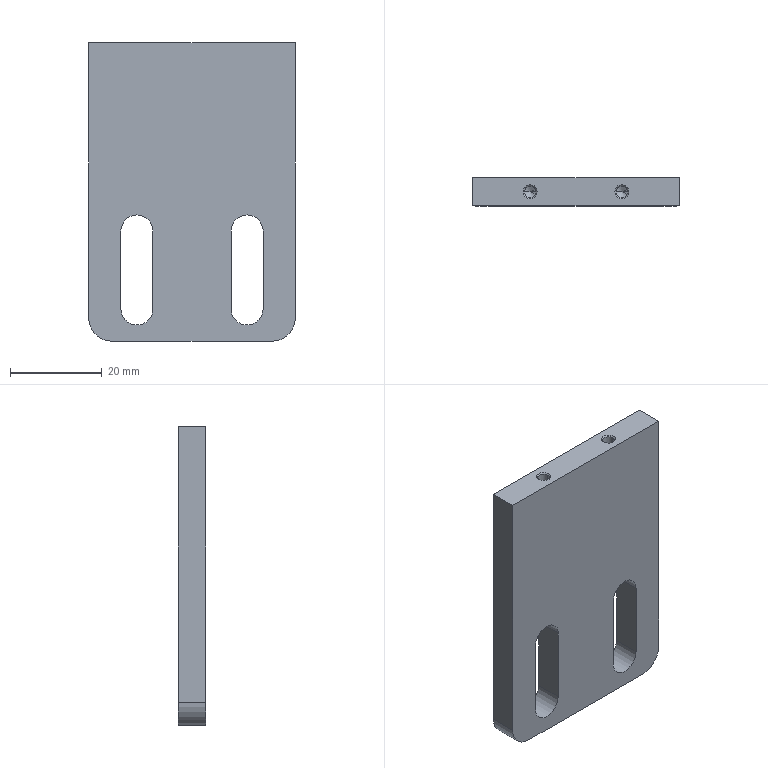Part | SolidWorks | features Extrusion 1, Fillet 1, HoleWzd 1, ICE 1 | 1 solid | 30 faces | box 45 x 6 x 65 mm | volume 15460 mm3 | cylinder 12 | plane 10 | cone 8 | commonest cylinder face diameters 7 x6 2.5 x4 10 x2
STEP:
#1=CARTESIAN_POINT('',(-11.25,3.,32.225));
#2=VERTEX_POINT('',#1);
#3=CARTESIAN_POINT('',(-8.75,3.,32.225));
#4=VERTEX_POINT('',#3);
#5=CARTESIAN_POINT('',(-10.,3.,32.225));
#6=DIRECTION('',(0.,0.,1.));
#7=DIRECTION('',(1.,0.,0.));
#8=AXIS2_PLACEMENT_3D('',#5,#6,#7);
#9=CIRCLE('',#8,1.25);
#10=EDGE_CURVE('',#2,#4,#9,.T.);
#11=ORIENTED_EDGE('',*,*,#10,.F.);
#12=CARTESIAN_POINT('',(-11.525,3.,32.5));
#13=VERTEX_POINT('',#12);
#14=CARTESIAN_POINT('',(-11.525,3.,32.5));
#15=DIRECTION('',(-0.7071,0.,0.7071));
#16=VECTOR('',#15,1000.);
#17=LINE('',#14,#16);
#18=EDGE_CURVE('',#2,#13,#17,.T.);
#19=ORIENTED_EDGE('',*,*,#18,.T.);
#20=CARTESIAN_POINT('',(-8.475,3.,32.5));
#21=VERTEX_POINT('',#20);
#22=CARTESIAN_POINT('',(-10.,3.,32.5));
#23=DIRECTION('',(0.,0.,1.));
#24=DIRECTION('',(1.,0.,0.));
#25=AXIS2_PLACEMENT_3D('',#22,#23,#24);
#26=CIRCLE('',#25,1.525);
#27=EDGE_CURVE('',#13,#21,#26,.T.);
#28=ORIENTED_EDGE('',*,*,#27,.T.);
#29=CARTESIAN_POINT('',(-8.475,3.,32.5));
#30=DIRECTION('',(0.7071,0.,0.7071));
#31=VECTOR('',#30,1000.);
#32=LINE('',#29,#31);
#33=EDGE_CURVE('',#4,#21,#32,.T.);
#34=ORIENTED_EDGE('',*,*,#33,.F.);
#35=EDGE_LOOP('',(#11,#19,#28,#34));
#36=FACE_OUTER_BOUND('',#35,.T.);
#37=CARTESIAN_POINT('',(-10.,3.,32.5));
#38=DIRECTION('',(0.,0.,1.));
#39=DIRECTION('',(1.,0.,0.));
#40=AXIS2_PLACEMENT_3D('',#37,#38,#39);
#41=CONICAL_SURFACE('',#40,1.525,0.7854);
#42=ADVANCED_FACE('',(#36),#41,.F.);
#43=CARTESIAN_POINT('',(-11.25,3.,19.));
#44=VERTEX_POINT('',#43);
#45=CARTESIAN_POINT('',(-8.75,3.,19.));
#46=VERTEX_POINT('',#45);
#47=CARTESIAN_POINT('',(-10.,3.,19.));
#48=DIRECTION('',(0.,0.,1.));
#49=DIRECTION('',(1.,0.,0.));
#50=AXIS2_PLACEMENT_3D('',#47,#48,#49);
#51=CIRCLE('',#50,1.25);
#52=EDGE_CURVE('',#44,#46,#51,.T.);
#53=ORIENTED_EDGE('',*,*,#52,.F.);
#54=CARTESIAN_POINT('',(-11.25,3.,32.5));
#55=DIRECTION('',(0.,0.,1.));
#56=VECTOR('',#55,1000.);
#57=LINE('',#54,#56);
#58=EDGE_CURVE('',#44,#2,#57,.T.);
#59=ORIENTED_EDGE('',*,*,#58,.T.);
#60=ORIENTED_EDGE('',*,*,#10,.T.);
#61=CARTESIAN_POINT('',(-8.75,3.,32.5));
#62=DIRECTION('',(0.,0.,1.));
#63=VECTOR('',#62,1000.);
#64=LINE('',#61,#63);
#65=EDGE_CURVE('',#46,#4,#64,.T.);
#66=ORIENTED_EDGE('',*,*,#65,.F.);
#67=EDGE_LOOP('',(#53,#59,#60,#66));
#68=FACE_OUTER_BOUND('',#67,.T.);
#69=CARTESIAN_POINT('',(-10.,3.,32.5));
#70=DIRECTION('',(0.,0.,1.));
#71=DIRECTION('',(1.,0.,0.));
#72=AXIS2_PLACEMENT_3D('',#69,#70,#71);
#73=CYLINDRICAL_SURFACE('',#72,1.25);
#74=ADVANCED_FACE('',(#68),#73,.F.);
#75=CARTESIAN_POINT('',(-10.,3.,18.249));
#76=VERTEX_POINT('',#75);
#77=CARTESIAN_POINT('',(-8.75,3.,19.));
#78=DIRECTION('',(0.8572,0.,0.515));
#79=VECTOR('',#78,1000.);
#80=LINE('',#77,#79);
#81=EDGE_CURVE('',#76,#46,#80,.T.);
#82=ORIENTED_EDGE('',*,*,#81,.F.);
#83=CARTESIAN_POINT('',(-11.25,3.,19.));
#84=DIRECTION('',(-0.8572,0.,0.515));
#85=VECTOR('',#84,1000.);
#86=LINE('',#83,#85);
#87=EDGE_CURVE('',#76,#44,#86,.T.);
#88=ORIENTED_EDGE('',*,*,#87,.T.);
#89=ORIENTED_EDGE('',*,*,#52,.T.);
#90=EDGE_LOOP('',(#82,#88,#89));
#91=FACE_OUTER_BOUND('',#90,.T.);
#92=CARTESIAN_POINT('',(-10.,3.,19.));
#93=DIRECTION('',(0.,0.,1.));
#94=DIRECTION('',(1.,0.,0.));
#95=AXIS2_PLACEMENT_3D('',#92,#93,#94);
#96=CONICAL_SURFACE('',#95,1.25,1.03);
#97=ADVANCED_FACE('',(#91),#96,.F.);
#98=CARTESIAN_POINT('',(8.75,3.,32.225));
#99=VERTEX_POINT('',#98);
#100=CARTESIAN_POINT('',(11.25,3.,32.225));
#101=VERTEX_POINT('',#100);
#102=CARTESIAN_POINT('',(10.,3.,32.225));
#103=DIRECTION('',(0.,0.,1.));
#104=DIRECTION('',(1.,0.,0.));
#105=AXIS2_PLACEMENT_3D('',#102,#103,#104);
#106=CIRCLE('',#105,1.25);
#107=EDGE_CURVE('',#99,#101,#106,.T.);
#108=ORIENTED_EDGE('',*,*,#107,.F.);
#109=CARTESIAN_POINT('',(8.475,3.,32.5));
#110=VERTEX_POINT('',#109);
#111=CARTESIAN_POINT('',(8.475,3.,32.5));
#112=DIRECTION('',(-0.7071,0.,0.7071));
#113=VECTOR('',#112,1000.);
#114=LINE('',#111,#113);
#115=EDGE_CURVE('',#99,#110,#114,.T.);
#116=ORIENTED_EDGE('',*,*,#115,.T.);
#117=CARTESIAN_POINT('',(11.525,3.,32.5));
#118=VERTEX_POINT('',#117);
#119=CARTESIAN_POINT('',(10.,3.,32.5));
#120=DIRECTION('',(0.,0.,1.));
#121=DIRECTION('',(1.,0.,0.));
#122=AXIS2_PLACEMENT_3D('',#119,#120,#121);
#123=CIRCLE('',#122,1.525);
#124=EDGE_CURVE('',#110,#118,#123,.T.);
#125=ORIENTED_EDGE('',*,*,#124,.T.);
#126=CARTESIAN_POINT('',(11.525,3.,32.5));
#127=DIRECTION('',(0.7071,0.,0.7071));
#128=VECTOR('',#127,1000.);
#129=LINE('',#126,#128);
#130=EDGE_CURVE('',#101,#118,#129,.T.);
#131=ORIENTED_EDGE('',*,*,#130,.F.);
#132=EDGE_LOOP('',(#108,#116,#125,#131));
#133=FACE_OUTER_BOUND('',#132,.T.);
#134=CARTESIAN_POINT('',(10.,3.,32.5));
#135=DIRECTION('',(0.,0.,1.));
#136=DIRECTION('',(1.,0.,0.));
#137=AXIS2_PLACEMENT_3D('',#134,#135,#136);
#138=CONICAL_SURFACE('',#137,1.525,0.7854);
#139=ADVANCED_FACE('',(#133),#138,.F.);
#140=CARTESIAN_POINT('',(8.75,3.,19.));
#141=VERTEX_POINT('',#140);
#142=CARTESIAN_POINT('',(11.25,3.,19.));
#143=VERTEX_POINT('',#142);
#144=CARTESIAN_POINT('',(10.,3.,19.));
#145=DIRECTION('',(0.,0.,1.));
#146=DIRECTION('',(1.,0.,0.));
#147=AXIS2_PLACEMENT_3D('',#144,#145,#146);
#148=CIRCLE('',#147,1.25);
#149=EDGE_CURVE('',#141,#143,#148,.T.);
#150=ORIENTED_EDGE('',*,*,#149,.F.);
#151=CARTESIAN_POINT('',(8.75,3.,32.5));
#152=DIRECTION('',(0.,0.,1.));
#153=VECTOR('',#152,1000.);
#154=LINE('',#151,#153);
#155=EDGE_CURVE('',#141,#99,#154,.T.);
#156=ORIENTED_EDGE('',*,*,#155,.T.);
#157=ORIENTED_EDGE('',*,*,#107,.T.);
#158=CARTESIAN_POINT('',(11.25,3.,32.5));
#159=DIRECTION('',(0.,0.,1.));
#160=VECTOR('',#159,1000.);
#161=LINE('',#158,#160);
#162=EDGE_CURVE('',#143,#101,#161,.T.);
#163=ORIENTED_EDGE('',*,*,#162,.F.);
#164=EDGE_LOOP('',(#150,#156,#157,#163));
#165=FACE_OUTER_BOUND('',#164,.T.);
#166=CARTESIAN_POINT('',(10.,3.,32.5));
#167=DIRECTION('',(0.,0.,1.));
#168=DIRECTION('',(1.,0.,0.));
#169=AXIS2_PLACEMENT_3D('',#166,#167,#168);
#170=CYLINDRICAL_SURFACE('',#169,1.25);
#171=ADVANCED_FACE('',(#165),#170,.F.);
#172=CARTESIAN_POINT('',(10.,3.,18.249));
#173=VERTEX_POINT('',#172);
#174=CARTESIAN_POINT('',(11.25,3.,19.));
#175=DIRECTION('',(0.8572,0.,0.515));
#176=VECTOR('',#175,1000.);
#177=LINE('',#174,#176);
#178=EDGE_CURVE('',#173,#143,#177,.T.);
#179=ORIENTED_EDGE('',*,*,#178,.F.);
#180=CARTESIAN_POINT('',(8.75,3.,19.));
#181=DIRECTION('',(-0.8572,0.,0.515));
#182=VECTOR('',#181,1000.);
#183=LINE('',#180,#182);
#184=EDGE_CURVE('',#173,#141,#183,.T.);
#185=ORIENTED_EDGE('',*,*,#184,.T.);
#186=ORIENTED_EDGE('',*,*,#149,.T.);
#187=EDGE_LOOP('',(#179,#185,#186));
#188=FACE_OUTER_BOUND('',#187,.T.);
#189=CARTESIAN_POINT('',(10.,3.,19.));
#190=DIRECTION('',(0.,0.,1.));
#191=DIRECTION('',(1.,0.,0.));
#192=AXIS2_PLACEMENT_3D('',#189,#190,#191);
#193=CONICAL_SURFACE('',#192,1.25,1.03);
#194=ADVANCED_FACE('',(#188),#193,.F.);
#195=CARTESIAN_POINT('',(-12.,0.,-5.));
#196=VERTEX_POINT('',#195);
#197=CARTESIAN_POINT('',(-8.5,0.,-8.5));
#198=VERTEX_POINT('',#197);
#199=CARTESIAN_POINT('',(-12.,0.,-8.5));
#200=DIRECTION('',(0.,1.,0.));
#201=DIRECTION('',(0.,0.,1.));
#202=AXIS2_PLACEMENT_3D('',#199,#200,#201);
#203=CIRCLE('',#202,3.5);
#204=EDGE_CURVE('',#196,#198,#203,.T.);
#205=ORIENTED_EDGE('',*,*,#204,.F.);
#206=CARTESIAN_POINT('',(-12.,6.,-5.));
#207=VERTEX_POINT('',#206);
#208=CARTESIAN_POINT('',(-12.,0.,-5.));
#209=DIRECTION('',(0.,1.,0.));
#210=VECTOR('',#209,1000.);
#211=LINE('',#208,#210);
#212=EDGE_CURVE('',#196,#207,#211,.T.);
#213=ORIENTED_EDGE('',*,*,#212,.T.);
#214=CARTESIAN_POINT('',(-8.5,6.,-8.5));
#215=VERTEX_POINT('',#214);
#216=CARTESIAN_POINT('',(-12.,6.,-8.5));
#217=DIRECTION('',(0.,1.,0.));
#218=DIRECTION('',(0.,0.,1.));
#219=AXIS2_PLACEMENT_3D('',#216,#217,#218);
#220=CIRCLE('',#219,3.5);
#221=EDGE_CURVE('',#207,#215,#220,.T.);
#222=ORIENTED_EDGE('',*,*,#221,.T.);
#223=CARTESIAN_POINT('',(-8.5,0.,-8.5));
#224=DIRECTION('',(0.,1.,0.));
#225=VECTOR('',#224,1000.);
#226=LINE('',#223,#225);
#227=EDGE_CURVE('',#198,#215,#226,.T.);
#228=ORIENTED_EDGE('',*,*,#227,.F.);
#229=EDGE_LOOP('',(#205,#213,#222,#228));
#230=FACE_OUTER_BOUND('',#229,.T.);
#231=CARTESIAN_POINT('',(-12.,0.,-8.5));
#232=DIRECTION('',(0.,1.,0.));
#233=DIRECTION('',(0.,0.,1.));
#234=AXIS2_PLACEMENT_3D('',#231,#232,#233);
#235=CYLINDRICAL_SURFACE('',#234,3.5);
#236=ADVANCED_FACE('',(#230),#235,.F.);
#237=CARTESIAN_POINT('',(12.,0.,-5.));
#238=VERTEX_POINT('',#237);
#239=CARTESIAN_POINT('',(15.5,0.,-8.5));
#240=VERTEX_POINT('',#239);
#241=CARTESIAN_POINT('',(12.,0.,-8.5));
#242=DIRECTION('',(0.,1.,0.));
#243=DIRECTION('',(0.,0.,-1.));
#244=AXIS2_PLACEMENT_3D('',#241,#242,#243);
#245=CIRCLE('',#244,3.5);
#246=EDGE_CURVE('',#238,#240,#245,.T.);
#247=ORIENTED_EDGE('',*,*,#246,.F.);
#248=CARTESIAN_POINT('',(12.,6.,-5.));
#249=VERTEX_POINT('',#248);
#250=CARTESIAN_POINT('',(12.,0.,-5.));
#251=DIRECTION('',(0.,1.,0.));
#252=VECTOR('',#251,1000.);
#253=LINE('',#250,#252);
#254=EDGE_CURVE('',#238,#249,#253,.T.);
#255=ORIENTED_EDGE('',*,*,#254,.T.);
#256=CARTESIAN_POINT('',(15.5,6.,-8.5));
#257=VERTEX_POINT('',#256);
#258=CARTESIAN_POINT('',(12.,6.,-8.5));
#259=DIRECTION('',(0.,1.,0.));
#260=DIRECTION('',(0.,0.,-1.));
#261=AXIS2_PLACEMENT_3D('',#258,#259,#260);
#262=CIRCLE('',#261,3.5);
#263=EDGE_CURVE('',#249,#257,#262,.T.);
#264=ORIENTED_EDGE('',*,*,#263,.T.);
#265=CARTESIAN_POINT('',(15.5,0.,-8.5));
#266=DIRECTION('',(0.,1.,0.));
#267=VECTOR('',#266,1000.);
#268=LINE('',#265,#267);
#269=EDGE_CURVE('',#240,#257,#268,.T.);
#270=ORIENTED_EDGE('',*,*,#269,.F.);
#271=EDGE_LOOP('',(#247,#255,#264,#270));
#272=FACE_OUTER_BOUND('',#271,.T.);
#273=CARTESIAN_POINT('',(12.,0.,-8.5));
#274=DIRECTION('',(0.,1.,0.));
#275=DIRECTION('',(0.,0.,1.));
#276=AXIS2_PLACEMENT_3D('',#273,#274,#275);
#277=CYLINDRICAL_SURFACE('',#276,3.5);
#278=ADVANCED_FACE('',(#272),#277,.F.);
#279=CARTESIAN_POINT('',(-22.5,6.,-27.5));
#280=VERTEX_POINT('',#279);
#281=CARTESIAN_POINT('',(-22.5,6.,32.5));
#282=VERTEX_POINT('',#281);
#283=CARTESIAN_POINT('',(-22.5,6.,32.5));
#284=DIRECTION('',(0.,0.,1.));
#285=VECTOR('',#284,1000.);
#286=LINE('',#283,#285);
#287=EDGE_CURVE('',#280,#282,#286,.T.);
#288=ORIENTED_EDGE('',*,*,#287,.F.);
#289=CARTESIAN_POINT('',(-22.5,0.,-27.5));
#290=VERTEX_POINT('',#289);
#291=CARTESIAN_POINT('',(-22.5,6.,-27.5));
#292=DIRECTION('',(0.,-1.,0.));
#293=VECTOR('',#292,1000.);
#294=LINE('',#291,#293);
#295=EDGE_CURVE('',#280,#290,#294,.T.);
#296=ORIENTED_EDGE('',*,*,#295,.T.);
#297=CARTESIAN_POINT('',(-22.5,0.,32.5));
#298=VERTEX_POINT('',#297);
#299=CARTESIAN_POINT('',(-22.5,0.,32.5));
#300=DIRECTION('',(0.,0.,1.));
#301=VECTOR('',#300,1000.);
#302=LINE('',#299,#301);
#303=EDGE_CURVE('',#290,#298,#302,.T.);
#304=ORIENTED_EDGE('',*,*,#303,.T.);
#305=CARTESIAN_POINT('',(-22.5,6.,32.5));
#306=DIRECTION('',(0.,-1.,0.));
#307=VECTOR('',#306,1000.);
#308=LINE('',#305,#307);
#309=EDGE_CURVE('',#282,#298,#308,.T.);
#310=ORIENTED_EDGE('',*,*,#309,.F.);
#311=EDGE_LOOP('',(#288,#296,#304,#310));
#312=FACE_OUTER_BOUND('',#311,.T.);
#313=CARTESIAN_POINT('',(-22.5,6.,32.5));
#314=DIRECTION('',(1.,0.,0.));
#315=DIRECTION('',(0.,0.,-1.));
#316=AXIS2_PLACEMENT_3D('',#313,#314,#315);
#317=PLANE('',#316);
#318=ADVANCED_FACE('',(#312),#317,.F.);
#319=CARTESIAN_POINT('',(-10.,3.,32.5));
#320=DIRECTION('',(0.,0.,1.));
#321=DIRECTION('',(1.,0.,0.));
#322=AXIS2_PLACEMENT_3D('',#319,#320,#321);
#323=CIRCLE('',#322,1.525);
#324=EDGE_CURVE('',#21,#13,#323,.T.);
#325=ORIENTED_EDGE('',*,*,#324,.F.);
#326=ORIENTED_EDGE('',*,*,#27,.F.);
#327=EDGE_LOOP('',(#325,#326));
#328=FACE_BOUND('',#327,.T.);
#329=CARTESIAN_POINT('',(10.,3.,32.5));
#330=DIRECTION('',(0.,0.,1.));
#331=DIRECTION('',(1.,0.,0.));
#332=AXIS2_PLACEMENT_3D('',#329,#330,#331);
#333=CIRCLE('',#332,1.525);
#334=EDGE_CURVE('',#118,#110,#333,.T.);
#335=ORIENTED_EDGE('',*,*,#334,.F.);
#336=ORIENTED_EDGE('',*,*,#124,.F.);
#337=EDGE_LOOP('',(#335,#336));
#338=FACE_BOUND('',#337,.T.);
#339=CARTESIAN_POINT('',(22.5,0.,32.5));
#340=VERTEX_POINT('',#339);
#341=CARTESIAN_POINT('',(22.5,0.,32.5));
#342=DIRECTION('',(1.,0.,0.));
#343=VECTOR('',#342,1000.);
#344=LINE('',#341,#343);
#345=EDGE_CURVE('',#298,#340,#344,.T.);
#346=ORIENTED_EDGE('',*,*,#345,.T.);
#347=CARTESIAN_POINT('',(22.5,6.,32.5));
#348=VERTEX_POINT('',#347);
#349=CARTESIAN_POINT('',(22.5,6.,32.5));
#350=DIRECTION('',(0.,-1.,0.));
#351=VECTOR('',#350,1000.);
#352=LINE('',#349,#351);
#353=EDGE_CURVE('',#348,#340,#352,.T.);
#354=ORIENTED_EDGE('',*,*,#353,.F.);
#355=CARTESIAN_POINT('',(22.5,6.,32.5));
#356=DIRECTION('',(1.,0.,0.));
#357=VECTOR('',#356,1000.);
#358=LINE('',#355,#357);
#359=EDGE_CURVE('',#282,#348,#358,.T.);
#360=ORIENTED_EDGE('',*,*,#359,.F.);
#361=ORIENTED_EDGE('',*,*,#309,.T.);
#362=EDGE_LOOP('',(#346,#354,#360,#361));
#363=FACE_OUTER_BOUND('',#362,.T.);
#364=CARTESIAN_POINT('',(22.5,6.,32.5));
#365=DIRECTION('',(0.,0.,-1.));
#366=DIRECTION('',(-1.,0.,0.));
#367=AXIS2_PLACEMENT_3D('',#364,#365,#366);
#368=PLANE('',#367);
#369=ADVANCED_FACE('',(#328,#338,#363),#368,.F.);
#370=CARTESIAN_POINT('',(22.5,0.,-27.5));
#371=VERTEX_POINT('',#370);
#372=CARTESIAN_POINT('',(22.5,0.,32.5));
#373=DIRECTION('',(0.,0.,-1.));
#374=VECTOR('',#373,1000.);
#375=LINE('',#372,#374);
#376=EDGE_CURVE('',#340,#371,#375,.T.);
#377=ORIENTED_EDGE('',*,*,#376,.T.);
#378=CARTESIAN_POINT('',(22.5,6.,-27.5));
#379=VERTEX_POINT('',#378);
#380=CARTESIAN_POINT('',(22.5,6.,-27.5));
#381=DIRECTION('',(0.,1.,0.));
#382=VECTOR('',#381,1000.);
#383=LINE('',#380,#382);
#384=EDGE_CURVE('',#371,#379,#383,.T.);
#385=ORIENTED_EDGE('',*,*,#384,.T.);
#386=CARTESIAN_POINT('',(22.5,6.,32.5));
#387=DIRECTION('',(0.,0.,-1.));
#388=VECTOR('',#387,1000.);
#389=LINE('',#386,#388);
#390=EDGE_CURVE('',#348,#379,#389,.T.);
#391=ORIENTED_EDGE('',*,*,#390,.F.);
#392=ORIENTED_EDGE('',*,*,#353,.T.);
#393=EDGE_LOOP('',(#377,#385,#391,#392));
#394=FACE_OUTER_BOUND('',#393,.T.);
#395=CARTESIAN_POINT('',(22.5,6.,32.5));
#396=DIRECTION('',(-1.,0.,0.));
#397=DIRECTION('',(0.,0.,1.));
#398=AXIS2_PLACEMENT_3D('',#395,#396,#397);
#399=PLANE('',#398);
#400=ADVANCED_FACE('',(#394),#399,.F.);
#401=CARTESIAN_POINT('',(17.5,6.,-32.5));
#402=VERTEX_POINT('',#401);
#403=CARTESIAN_POINT('',(-17.5,6.,-32.5));
#404=VERTEX_POINT('',#403);
#405=CARTESIAN_POINT('',(22.5,6.,-32.5));
#406=DIRECTION('',(-1.,0.,0.));
#407=VECTOR('',#406,1000.);
#408=LINE('',#405,#407);
#409=EDGE_CURVE('',#402,#404,#408,.T.);
#410=ORIENTED_EDGE('',*,*,#409,.F.);
#411=CARTESIAN_POINT('',(17.5,0.,-32.5));
#412=VERTEX_POINT('',#411);
#413=CARTESIAN_POINT('',(17.5,6.,-32.5));
#414=DIRECTION('',(0.,-1.,0.));
#415=VECTOR('',#414,1000.);
#416=LINE('',#413,#415);
#417=EDGE_CURVE('',#402,#412,#416,.T.);
#418=ORIENTED_EDGE('',*,*,#417,.T.);
#419=CARTESIAN_POINT('',(-17.5,0.,-32.5));
#420=VERTEX_POINT('',#419);
#421=CARTESIAN_POINT('',(22.5,0.,-32.5));
#422=DIRECTION('',(-1.,0.,0.));
#423=VECTOR('',#422,1000.);
#424=LINE('',#421,#423);
#425=EDGE_CURVE('',#412,#420,#424,.T.);
#426=ORIENTED_EDGE('',*,*,#425,.T.);
#427=CARTESIAN_POINT('',(-17.5,6.,-32.5));
#428=DIRECTION('',(0.,1.,0.));
#429=VECTOR('',#428,1000.);
#430=LINE('',#427,#429);
#431=EDGE_CURVE('',#420,#404,#430,.T.);
#432=ORIENTED_EDGE('',*,*,#431,.T.);
#433=EDGE_LOOP('',(#410,#418,#426,#432));
#434=FACE_OUTER_BOUND('',#433,.T.);
#435=CARTESIAN_POINT('',(22.5,6.,-32.5));
#436=DIRECTION('',(0.,0.,1.));
#437=DIRECTION('',(1.,0.,0.));
#438=AXIS2_PLACEMENT_3D('',#435,#436,#437);
#439=PLANE('',#438);
#440=ADVANCED_FACE('',(#434),#439,.F.);
#441=CARTESIAN_POINT('',(-8.5,6.,-25.5));
#442=VERTEX_POINT('',#441);
#443=CARTESIAN_POINT('',(-15.5,6.,-25.5));
#444=VERTEX_POINT('',#443);
#445=CARTESIAN_POINT('',(-12.,6.,-25.5));
#446=DIRECTION('',(0.,1.,0.));
#447=DIRECTION('',(0.,0.,1.));
#448=AXIS2_PLACEMENT_3D('',#445,#446,#447);
#449=CIRCLE('',#448,3.5);
#450=EDGE_CURVE('',#442,#444,#449,.T.);
#451=ORIENTED_EDGE('',*,*,#450,.F.);
#452=CARTESIAN_POINT('',(-8.5,6.,-25.5));
#453=DIRECTION('',(0.,0.,-1.));
#454=VECTOR('',#453,1000.);
#455=LINE('',#452,#454);
#456=EDGE_CURVE('',#215,#442,#455,.T.);
#457=ORIENTED_EDGE('',*,*,#456,.F.);
#458=ORIENTED_EDGE('',*,*,#221,.F.);
#459=CARTESIAN_POINT('',(-15.5,6.,-8.5));
#460=VERTEX_POINT('',#459);
#461=CARTESIAN_POINT('',(-12.,6.,-8.5));
#462=DIRECTION('',(0.,1.,0.));
#463=DIRECTION('',(0.,0.,1.));
#464=AXIS2_PLACEMENT_3D('',#461,#462,#463);
#465=CIRCLE('',#464,3.5);
#466=EDGE_CURVE('',#460,#207,#465,.T.);
#467=ORIENTED_EDGE('',*,*,#466,.F.);
#468=CARTESIAN_POINT('',(-15.5,6.,-25.5));
#469=DIRECTION('',(0.,0.,1.));
#470=VECTOR('',#469,1000.);
#471=LINE('',#468,#470);
#472=EDGE_CURVE('',#444,#460,#471,.T.);
#473=ORIENTED_EDGE('',*,*,#472,.F.);
#474=EDGE_LOOP('',(#451,#457,#458,#467,#473));
#475=FACE_BOUND('',#474,.T.);
#476=CARTESIAN_POINT('',(15.5,6.,-25.5));
#477=VERTEX_POINT('',#476);
#478=CARTESIAN_POINT('',(8.5,6.,-25.5));
#479=VERTEX_POINT('',#478);
#480=CARTESIAN_POINT('',(12.,6.,-25.5));
#481=DIRECTION('',(0.,1.,0.));
#482=DIRECTION('',(0.,0.,-1.));
#483=AXIS2_PLACEMENT_3D('',#480,#481,#482);
#484=CIRCLE('',#483,3.5);
#485=EDGE_CURVE('',#477,#479,#484,.T.);
#486=ORIENTED_EDGE('',*,*,#485,.F.);
#487=CARTESIAN_POINT('',(15.5,6.,-25.5));
#488=DIRECTION('',(0.,0.,-1.));
#489=VECTOR('',#488,1000.);
#490=LINE('',#487,#489);
#491=EDGE_CURVE('',#257,#477,#490,.T.);
#492=ORIENTED_EDGE('',*,*,#491,.F.);
#493=ORIENTED_EDGE('',*,*,#263,.F.);
#494=CARTESIAN_POINT('',(8.5,6.,-8.5));
#495=VERTEX_POINT('',#494);
#496=CARTESIAN_POINT('',(12.,6.,-8.5));
#497=DIRECTION('',(0.,1.,0.));
#498=DIRECTION('',(0.,0.,-1.));
#499=AXIS2_PLACEMENT_3D('',#496,#497,#498);
#500=CIRCLE('',#499,3.5);
#501=EDGE_CURVE('',#495,#249,#500,.T.);
#502=ORIENTED_EDGE('',*,*,#501,.F.);
#503=CARTESIAN_POINT('',(8.5,6.,-25.5));
#504=DIRECTION('',(0.,0.,1.));
#505=VECTOR('',#504,1000.);
#506=LINE('',#503,#505);
#507=EDGE_CURVE('',#479,#495,#506,.T.);
#508=ORIENTED_EDGE('',*,*,#507,.F.);
#509=EDGE_LOOP('',(#486,#492,#493,#502,#508));
#510=FACE_BOUND('',#509,.T.);
#511=ORIENTED_EDGE('',*,*,#390,.T.);
#512=CARTESIAN_POINT('',(17.5,6.,-27.5));
#513=DIRECTION('',(0.,1.,0.));
#514=DIRECTION('',(0.,0.,1.));
#515=AXIS2_PLACEMENT_3D('',#512,#513,#514);
#516=CIRCLE('',#515,5.);
#517=EDGE_CURVE('',#379,#402,#516,.T.);
#518=ORIENTED_EDGE('',*,*,#517,.T.);
#519=ORIENTED_EDGE('',*,*,#409,.T.);
#520=CARTESIAN_POINT('',(-17.5,6.,-27.5));
#521=DIRECTION('',(0.,1.,0.));
#522=DIRECTION('',(0.,0.,1.));
#523=AXIS2_PLACEMENT_3D('',#520,#521,#522);
#524=CIRCLE('',#523,5.);
#525=EDGE_CURVE('',#404,#280,#524,.T.);
#526=ORIENTED_EDGE('',*,*,#525,.T.);
#527=ORIENTED_EDGE('',*,*,#287,.T.);
#528=ORIENTED_EDGE('',*,*,#359,.T.);
#529=EDGE_LOOP('',(#511,#518,#519,#526,#527,#528));
#530=FACE_OUTER_BOUND('',#529,.T.);
#531=CARTESIAN_POINT('',(0.,6.,0.));
#532=DIRECTION('',(0.,1.,0.));
#533=DIRECTION('',(0.,0.,1.));
#534=AXIS2_PLACEMENT_3D('',#531,#532,#533);
#535=PLANE('',#534);
#536=ADVANCED_FACE('',(#475,#510,#530),#535,.T.);
#537=CARTESIAN_POINT('',(-8.5,0.,-25.5));
#538=VERTEX_POINT('',#537);
#539=CARTESIAN_POINT('',(-8.5,0.,-25.5));
#540=DIRECTION('',(0.,0.,-1.));
#541=VECTOR('',#540,1000.);
#542=LINE('',#539,#541);
#543=EDGE_CURVE('',#198,#538,#542,.T.);
#544=ORIENTED_EDGE('',*,*,#543,.T.);
#545=CARTESIAN_POINT('',(-15.5,0.,-25.5));
#546=VERTEX_POINT('',#545);
#547=CARTESIAN_POINT('',(-12.,0.,-25.5));
#548=DIRECTION('',(0.,1.,0.));
#549=DIRECTION('',(0.,0.,1.));
#550=AXIS2_PLACEMENT_3D('',#547,#548,#549);
#551=CIRCLE('',#550,3.5);
#552=EDGE_CURVE('',#538,#546,#551,.T.);
#553=ORIENTED_EDGE('',*,*,#552,.T.);
#554=CARTESIAN_POINT('',(-15.5,0.,-8.5));
#555=VERTEX_POINT('',#554);
#556=CARTESIAN_POINT('',(-15.5,0.,-25.5));
#557=DIRECTION('',(0.,0.,1.));
#558=VECTOR('',#557,1000.);
#559=LINE('',#556,#558);
#560=EDGE_CURVE('',#546,#555,#559,.T.);
#561=ORIENTED_EDGE('',*,*,#560,.T.);
#562=CARTESIAN_POINT('',(-12.,0.,-8.5));
#563=DIRECTION('',(0.,1.,0.));
#564=DIRECTION('',(0.,0.,1.));
#565=AXIS2_PLACEMENT_3D('',#562,#563,#564);
#566=CIRCLE('',#565,3.5);
#567=EDGE_CURVE('',#555,#196,#566,.T.);
#568=ORIENTED_EDGE('',*,*,#567,.T.);
#569=ORIENTED_EDGE('',*,*,#204,.T.);
#570=EDGE_LOOP('',(#544,#553,#561,#568,#569));
#571=FACE_BOUND('',#570,.T.);
#572=CARTESIAN_POINT('',(15.5,0.,-25.5));
#573=VERTEX_POINT('',#572);
#574=CARTESIAN_POINT('',(15.5,0.,-25.5));
#575=DIRECTION('',(0.,0.,-1.));
#576=VECTOR('',#575,1000.);
#577=LINE('',#574,#576);
#578=EDGE_CURVE('',#240,#573,#577,.T.);
#579=ORIENTED_EDGE('',*,*,#578,.T.);
#580=CARTESIAN_POINT('',(8.5,0.,-25.5));
#581=VERTEX_POINT('',#580);
#582=CARTESIAN_POINT('',(12.,0.,-25.5));
#583=DIRECTION('',(0.,1.,0.));
#584=DIRECTION('',(0.,0.,-1.));
#585=AXIS2_PLACEMENT_3D('',#582,#583,#584);
#586=CIRCLE('',#585,3.5);
#587=EDGE_CURVE('',#573,#581,#586,.T.);
#588=ORIENTED_EDGE('',*,*,#587,.T.);
#589=CARTESIAN_POINT('',(8.5,0.,-8.5));
#590=VERTEX_POINT('',#589);
#591=CARTESIAN_POINT('',(8.5,0.,-25.5));
#592=DIRECTION('',(0.,0.,1.));
#593=VECTOR('',#592,1000.);
#594=LINE('',#591,#593);
#595=EDGE_CURVE('',#581,#590,#594,.T.);
#596=ORIENTED_EDGE('',*,*,#595,.T.);
#597=CARTESIAN_POINT('',(12.,0.,-8.5));
#598=DIRECTION('',(0.,1.,0.));
#599=DIRECTION('',(0.,0.,-1.));
#600=AXIS2_PLACEMENT_3D('',#597,#598,#599);
#601=CIRCLE('',#600,3.5);
#602=EDGE_CURVE('',#590,#238,#601,.T.);
#603=ORIENTED_EDGE('',*,*,#602,.T.);
#604=ORIENTED_EDGE('',*,*,#246,.T.);
#605=EDGE_LOOP('',(#579,#588,#596,#603,#604));
#606=FACE_BOUND('',#605,.T.);
#607=ORIENTED_EDGE('',*,*,#425,.F.);
#608=CARTESIAN_POINT('',(17.5,0.,-27.5));
#609=DIRECTION('',(0.,-1.,0.));
#610=DIRECTION('',(0.,0.,1.));
#611=AXIS2_PLACEMENT_3D('',#608,#609,#610);
#612=CIRCLE('',#611,5.);
#613=EDGE_CURVE('',#412,#371,#612,.T.);
#614=ORIENTED_EDGE('',*,*,#613,.T.);
#615=ORIENTED_EDGE('',*,*,#376,.F.);
#616=ORIENTED_EDGE('',*,*,#345,.F.);
#617=ORIENTED_EDGE('',*,*,#303,.F.);
#618=CARTESIAN_POINT('',(-17.5,0.,-27.5));
#619=DIRECTION('',(0.,-1.,0.));
#620=DIRECTION('',(0.,0.,1.));
#621=AXIS2_PLACEMENT_3D('',#618,#619,#620);
#622=CIRCLE('',#621,5.);
#623=EDGE_CURVE('',#290,#420,#622,.T.);
#624=ORIENTED_EDGE('',*,*,#623,.T.);
#625=EDGE_LOOP('',(#607,#614,#615,#616,#617,#624));
#626=FACE_OUTER_BOUND('',#625,.T.);
#627=CARTESIAN_POINT('',(0.,0.,0.));
#628=DIRECTION('',(0.,1.,0.));
#629=DIRECTION('',(0.,0.,1.));
#630=AXIS2_PLACEMENT_3D('',#627,#628,#629);
#631=PLANE('',#630);
#632=ADVANCED_FACE('',(#571,#606,#626),#631,.F.);
#633=ORIENTED_EDGE('',*,*,#485,.T.);
#634=CARTESIAN_POINT('',(8.5,0.,-25.5));
#635=DIRECTION('',(0.,1.,0.));
#636=VECTOR('',#635,1000.);
#637=LINE('',#634,#636);
#638=EDGE_CURVE('',#581,#479,#637,.T.);
#639=ORIENTED_EDGE('',*,*,#638,.F.);
#640=ORIENTED_EDGE('',*,*,#587,.F.);
#641=CARTESIAN_POINT('',(15.5,0.,-25.5));
#642=DIRECTION('',(0.,1.,0.));
#643=VECTOR('',#642,1000.);
#644=LINE('',#641,#643);
#645=EDGE_CURVE('',#573,#477,#644,.T.);
#646=ORIENTED_EDGE('',*,*,#645,.T.);
#647=EDGE_LOOP('',(#633,#639,#640,#646));
#648=FACE_OUTER_BOUND('',#647,.T.);
#649=CARTESIAN_POINT('',(12.,0.,-25.5));
#650=DIRECTION('',(0.,1.,0.));
#651=DIRECTION('',(0.,0.,1.));
#652=AXIS2_PLACEMENT_3D('',#649,#650,#651);
#653=CYLINDRICAL_SURFACE('',#652,3.5);
#654=ADVANCED_FACE('',(#648),#653,.F.);
#655=ORIENTED_EDGE('',*,*,#491,.T.);
#656=ORIENTED_EDGE('',*,*,#645,.F.);
#657=ORIENTED_EDGE('',*,*,#578,.F.);
#658=ORIENTED_EDGE('',*,*,#269,.T.);
#659=EDGE_LOOP('',(#655,#656,#657,#658));
#660=FACE_OUTER_BOUND('',#659,.T.);
#661=CARTESIAN_POINT('',(15.5,0.,-25.5));
#662=DIRECTION('',(1.,0.,0.));
#663=DIRECTION('',(0.,0.,-1.));
#664=AXIS2_PLACEMENT_3D('',#661,#662,#663);
#665=PLANE('',#664);
#666=ADVANCED_FACE('',(#660),#665,.F.);
#667=ORIENTED_EDGE('',*,*,#254,.F.);
#668=ORIENTED_EDGE('',*,*,#602,.F.);
#669=CARTESIAN_POINT('',(8.5,0.,-8.5));
#670=DIRECTION('',(0.,1.,0.));
#671=VECTOR('',#670,1000.);
#672=LINE('',#669,#671);
#673=EDGE_CURVE('',#590,#495,#672,.T.);
#674=ORIENTED_EDGE('',*,*,#673,.T.);
#675=ORIENTED_EDGE('',*,*,#501,.T.);
#676=EDGE_LOOP('',(#667,#668,#674,#675));
#677=FACE_OUTER_BOUND('',#676,.T.);
#678=CARTESIAN_POINT('',(12.,0.,-8.5));
#679=DIRECTION('',(0.,1.,0.));
#680=DIRECTION('',(0.,0.,1.));
#681=AXIS2_PLACEMENT_3D('',#678,#679,#680);
#682=CYLINDRICAL_SURFACE('',#681,3.5);
#683=ADVANCED_FACE('',(#677),#682,.F.);
#684=ORIENTED_EDGE('',*,*,#507,.T.);
#685=ORIENTED_EDGE('',*,*,#673,.F.);
#686=ORIENTED_EDGE('',*,*,#595,.F.);
#687=ORIENTED_EDGE('',*,*,#638,.T.);
#688=EDGE_LOOP('',(#684,#685,#686,#687));
#689=FACE_OUTER_BOUND('',#688,.T.);
#690=CARTESIAN_POINT('',(8.5,0.,-25.5));
#691=DIRECTION('',(-1.,0.,0.));
#692=DIRECTION('',(0.,0.,1.));
#693=AXIS2_PLACEMENT_3D('',#690,#691,#692);
#694=PLANE('',#693);
#695=ADVANCED_FACE('',(#689),#694,.F.);
#696=ORIENTED_EDGE('',*,*,#450,.T.);
#697=CARTESIAN_POINT('',(-15.5,0.,-25.5));
#698=DIRECTION('',(0.,1.,0.));
#699=VECTOR('',#698,1000.);
#700=LINE('',#697,#699);
#701=EDGE_CURVE('',#546,#444,#700,.T.);
#702=ORIENTED_EDGE('',*,*,#701,.F.);
#703=ORIENTED_EDGE('',*,*,#552,.F.);
#704=CARTESIAN_POINT('',(-8.5,0.,-25.5));
#705=DIRECTION('',(0.,1.,0.));
#706=VECTOR('',#705,1000.);
#707=LINE('',#704,#706);
#708=EDGE_CURVE('',#538,#442,#707,.T.);
#709=ORIENTED_EDGE('',*,*,#708,.T.);
#710=EDGE_LOOP('',(#696,#702,#703,#709));
#711=FACE_OUTER_BOUND('',#710,.T.);
#712=CARTESIAN_POINT('',(-12.,0.,-25.5));
#713=DIRECTION('',(0.,1.,0.));
#714=DIRECTION('',(0.,0.,1.));
#715=AXIS2_PLACEMENT_3D('',#712,#713,#714);
#716=CYLINDRICAL_SURFACE('',#715,3.5);
#717=ADVANCED_FACE('',(#711),#716,.F.);
#718=ORIENTED_EDGE('',*,*,#456,.T.);
#719=ORIENTED_EDGE('',*,*,#708,.F.);
#720=ORIENTED_EDGE('',*,*,#543,.F.);
#721=ORIENTED_EDGE('',*,*,#227,.T.);
#722=EDGE_LOOP('',(#718,#719,#720,#721));
#723=FACE_OUTER_BOUND('',#722,.T.);
#724=CARTESIAN_POINT('',(-8.5,0.,-25.5));
#725=DIRECTION('',(1.,0.,0.));
#726=DIRECTION('',(0.,0.,-1.));
#727=AXIS2_PLACEMENT_3D('',#724,#725,#726);
#728=PLANE('',#727);
#729=ADVANCED_FACE('',(#723),#728,.F.);
#730=ORIENTED_EDGE('',*,*,#212,.F.);
#731=ORIENTED_EDGE('',*,*,#567,.F.);
#732=CARTESIAN_POINT('',(-15.5,0.,-8.5));
#733=DIRECTION('',(0.,1.,0.));
#734=VECTOR('',#733,1000.);
#735=LINE('',#732,#734);
#736=EDGE_CURVE('',#555,#460,#735,.T.);
#737=ORIENTED_EDGE('',*,*,#736,.T.);
#738=ORIENTED_EDGE('',*,*,#466,.T.);
#739=EDGE_LOOP('',(#730,#731,#737,#738));
#740=FACE_OUTER_BOUND('',#739,.T.);
#741=CARTESIAN_POINT('',(-12.,0.,-8.5));
#742=DIRECTION('',(0.,1.,0.));
#743=DIRECTION('',(0.,0.,1.));
#744=AXIS2_PLACEMENT_3D('',#741,#742,#743);
#745=CYLINDRICAL_SURFACE('',#744,3.5);
#746=ADVANCED_FACE('',(#740),#745,.F.);
#747=ORIENTED_EDGE('',*,*,#472,.T.);
#748=ORIENTED_EDGE('',*,*,#736,.F.);
#749=ORIENTED_EDGE('',*,*,#560,.F.);
#750=ORIENTED_EDGE('',*,*,#701,.T.);
#751=EDGE_LOOP('',(#747,#748,#749,#750));
#752=FACE_OUTER_BOUND('',#751,.T.);
#753=CARTESIAN_POINT('',(-15.5,0.,-25.5));
#754=DIRECTION('',(-1.,0.,0.));
#755=DIRECTION('',(0.,0.,1.));
#756=AXIS2_PLACEMENT_3D('',#753,#754,#755);
#757=PLANE('',#756);
#758=ADVANCED_FACE('',(#752),#757,.F.);
#759=ORIENTED_EDGE('',*,*,#517,.F.);
#760=ORIENTED_EDGE('',*,*,#384,.F.);
#761=ORIENTED_EDGE('',*,*,#613,.F.);
#762=ORIENTED_EDGE('',*,*,#417,.F.);
#763=EDGE_LOOP('',(#759,#760,#761,#762));
#764=FACE_OUTER_BOUND('',#763,.T.);
#765=CARTESIAN_POINT('',(17.5,6.,-27.5));
#766=DIRECTION('',(0.,-1.,0.));
#767=DIRECTION('',(0.,0.,-1.));
#768=AXIS2_PLACEMENT_3D('',#765,#766,#767);
#769=CYLINDRICAL_SURFACE('',#768,5.);
#770=ADVANCED_FACE('',(#764),#769,.T.);
#771=ORIENTED_EDGE('',*,*,#525,.F.);
#772=ORIENTED_EDGE('',*,*,#431,.F.);
#773=ORIENTED_EDGE('',*,*,#623,.F.);
#774=ORIENTED_EDGE('',*,*,#295,.F.);
#775=EDGE_LOOP('',(#771,#772,#773,#774));
#776=FACE_OUTER_BOUND('',#775,.T.);
#777=CARTESIAN_POINT('',(-17.5,6.,-27.5));
#778=DIRECTION('',(0.,-1.,0.));
#779=DIRECTION('',(0.,0.,-1.));
#780=AXIS2_PLACEMENT_3D('',#777,#778,#779);
#781=CYLINDRICAL_SURFACE('',#780,5.);
#782=ADVANCED_FACE('',(#776),#781,.T.);
#783=ORIENTED_EDGE('',*,*,#184,.F.);
#784=ORIENTED_EDGE('',*,*,#178,.T.);
#785=CARTESIAN_POINT('',(10.,3.,19.));
#786=DIRECTION('',(0.,0.,1.));
#787=DIRECTION('',(1.,0.,0.));
#788=AXIS2_PLACEMENT_3D('',#785,#786,#787);
#789=CIRCLE('',#788,1.25);
#790=EDGE_CURVE('',#143,#141,#789,.T.);
#791=ORIENTED_EDGE('',*,*,#790,.T.);
#792=EDGE_LOOP('',(#783,#784,#791));
#793=FACE_OUTER_BOUND('',#792,.T.);
#794=CARTESIAN_POINT('',(10.,3.,19.));
#795=DIRECTION('',(0.,0.,1.));
#796=DIRECTION('',(1.,0.,0.));
#797=AXIS2_PLACEMENT_3D('',#794,#795,#796);
#798=CONICAL_SURFACE('',#797,1.25,1.03);
#799=ADVANCED_FACE('',(#793),#798,.F.);
#800=ORIENTED_EDGE('',*,*,#155,.F.);
#801=ORIENTED_EDGE('',*,*,#790,.F.);
#802=ORIENTED_EDGE('',*,*,#162,.T.);
#803=CARTESIAN_POINT('',(10.,3.,32.225));
#804=DIRECTION('',(0.,0.,1.));
#805=DIRECTION('',(1.,0.,0.));
#806=AXIS2_PLACEMENT_3D('',#803,#804,#805);
#807=CIRCLE('',#806,1.25);
#808=EDGE_CURVE('',#101,#99,#807,.T.);
#809=ORIENTED_EDGE('',*,*,#808,.T.);
#810=EDGE_LOOP('',(#800,#801,#802,#809));
#811=FACE_OUTER_BOUND('',#810,.T.);
#812=CARTESIAN_POINT('',(10.,3.,32.5));
#813=DIRECTION('',(0.,0.,1.));
#814=DIRECTION('',(1.,0.,0.));
#815=AXIS2_PLACEMENT_3D('',#812,#813,#814);
#816=CYLINDRICAL_SURFACE('',#815,1.25);
#817=ADVANCED_FACE('',(#811),#816,.F.);
#818=ORIENTED_EDGE('',*,*,#115,.F.);
#819=ORIENTED_EDGE('',*,*,#808,.F.);
#820=ORIENTED_EDGE('',*,*,#130,.T.);
#821=ORIENTED_EDGE('',*,*,#334,.T.);
#822=EDGE_LOOP('',(#818,#819,#820,#821));
#823=FACE_OUTER_BOUND('',#822,.T.);
#824=CARTESIAN_POINT('',(10.,3.,32.5));
#825=DIRECTION('',(0.,0.,1.));
#826=DIRECTION('',(1.,0.,0.));
#827=AXIS2_PLACEMENT_3D('',#824,#825,#826);
#828=CONICAL_SURFACE('',#827,1.525,0.7854);
#829=ADVANCED_FACE('',(#823),#828,.F.);
#830=ORIENTED_EDGE('',*,*,#87,.F.);
#831=ORIENTED_EDGE('',*,*,#81,.T.);
#832=CARTESIAN_POINT('',(-10.,3.,19.));
#833=DIRECTION('',(0.,0.,1.));
#834=DIRECTION('',(1.,0.,0.));
#835=AXIS2_PLACEMENT_3D('',#832,#833,#834);
#836=CIRCLE('',#835,1.25);
#837=EDGE_CURVE('',#46,#44,#836,.T.);
#838=ORIENTED_EDGE('',*,*,#837,.T.);
#839=EDGE_LOOP('',(#830,#831,#838));
#840=FACE_OUTER_BOUND('',#839,.T.);
#841=CARTESIAN_POINT('',(-10.,3.,19.));
#842=DIRECTION('',(0.,0.,1.));
#843=DIRECTION('',(1.,0.,0.));
#844=AXIS2_PLACEMENT_3D('',#841,#842,#843);
#845=CONICAL_SURFACE('',#844,1.25,1.03);
#846=ADVANCED_FACE('',(#840),#845,.F.);
#847=ORIENTED_EDGE('',*,*,#58,.F.);
#848=ORIENTED_EDGE('',*,*,#837,.F.);
#849=ORIENTED_EDGE('',*,*,#65,.T.);
#850=CARTESIAN_POINT('',(-10.,3.,32.225));
#851=DIRECTION('',(0.,0.,1.));
#852=DIRECTION('',(1.,0.,0.));
#853=AXIS2_PLACEMENT_3D('',#850,#851,#852);
#854=CIRCLE('',#853,1.25);
#855=EDGE_CURVE('',#4,#2,#854,.T.);
#856=ORIENTED_EDGE('',*,*,#855,.T.);
#857=EDGE_LOOP('',(#847,#848,#849,#856));
#858=FACE_OUTER_BOUND('',#857,.T.);
#859=CARTESIAN_POINT('',(-10.,3.,32.5));
#860=DIRECTION('',(0.,0.,1.));
#861=DIRECTION('',(1.,0.,0.));
#862=AXIS2_PLACEMENT_3D('',#859,#860,#861);
#863=CYLINDRICAL_SURFACE('',#862,1.25);
#864=ADVANCED_FACE('',(#858),#863,.F.);
#865=ORIENTED_EDGE('',*,*,#18,.F.);
#866=ORIENTED_EDGE('',*,*,#855,.F.);
#867=ORIENTED_EDGE('',*,*,#33,.T.);
#868=ORIENTED_EDGE('',*,*,#324,.T.);
#869=EDGE_LOOP('',(#865,#866,#867,#868));
#870=FACE_OUTER_BOUND('',#869,.T.);
#871=CARTESIAN_POINT('',(-10.,3.,32.5));
#872=DIRECTION('',(0.,0.,1.));
#873=DIRECTION('',(1.,0.,0.));
#874=AXIS2_PLACEMENT_3D('',#871,#872,#873);
#875=CONICAL_SURFACE('',#874,1.525,0.7854);
#876=ADVANCED_FACE('',(#870),#875,.F.);
#877=CLOSED_SHELL('',(#42,#74,#97,#139,#171,#194,#236,#278,#318,#369,#400,#440,#536,#632,#654,#666,#683,#695,#717,#729,#746,#758,#770,#782,#799,#817,#829,#846,#864,#876));
#878=MANIFOLD_SOLID_BREP('',#877);
#879=CARTESIAN_POINT('',(0.,0.,0.));
#880=DIRECTION('',(0.,0.,1.));
#881=DIRECTION('',(1.,0.,0.));
#882=AXIS2_PLACEMENT_3D('',#879,#880,#881);
#883=(LENGTH_UNIT()NAMED_UNIT(*)SI_UNIT(.MILLI.,.METRE.));
#884=UNCERTAINTY_MEASURE_WITH_UNIT(LENGTH_MEASURE(0.00001),#883,'','');
#885=(NAMED_UNIT(*)PLANE_ANGLE_UNIT()SI_UNIT($,.RADIAN.));
#886=(NAMED_UNIT(*)SI_UNIT($,.STERADIAN.)SOLID_ANGLE_UNIT());
#887=(GEOMETRIC_REPRESENTATION_CONTEXT(3)GLOBAL_UNCERTAINTY_ASSIGNED_CONTEXT((#884))GLOBAL_UNIT_ASSIGNED_CONTEXT((#883,#885,#886))REPRESENTATION_CONTEXT('',''));
#888=ADVANCED_BREP_SHAPE_REPRESENTATION('',(#878,#882),#887);